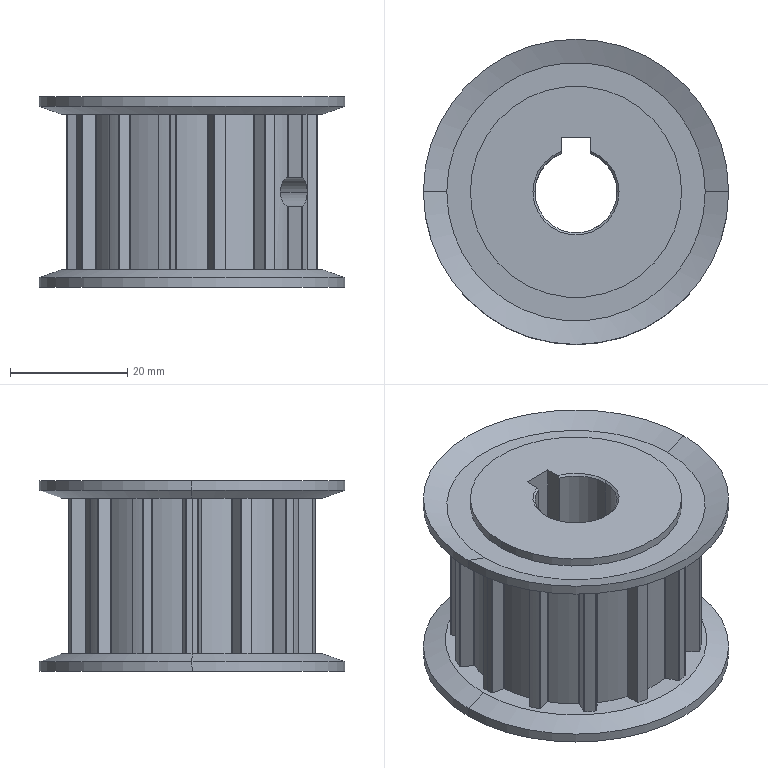Part | SolidWorks | features ICE 10, Chamfer 9, RevCut 3, CirPattern 2, Revolution 2 | 1 solid | 167 faces | box 52 x 52 x 32.5 mm | volume 36076 mm3 | cylinder 114 | plane 39 | cone 14 | commonest cylinder face diameters 0.2 x70 42.7 x15 37.98 x14 5 x4 36 x4 52 x4